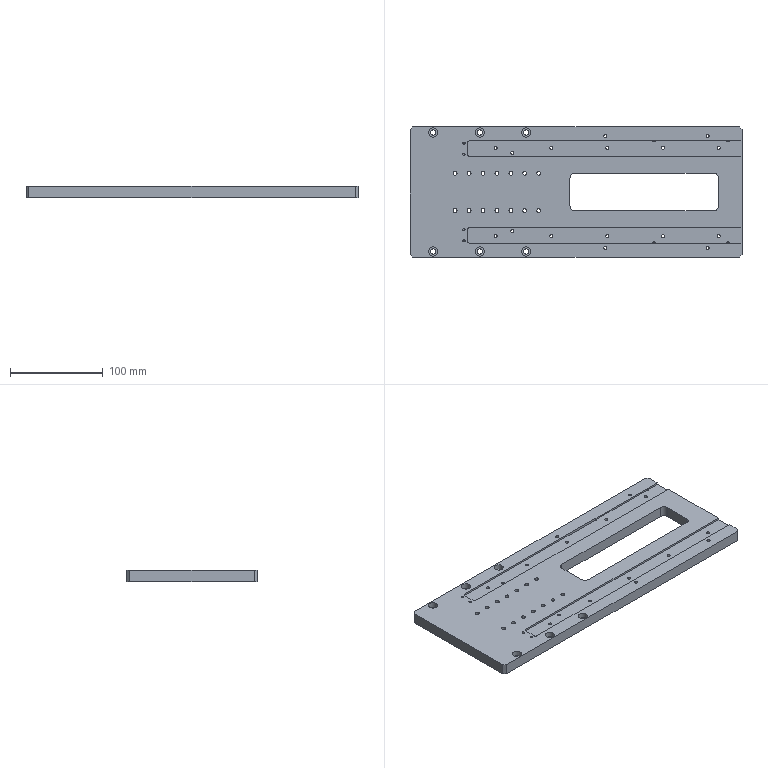Part | 1 solid | 105 faces | box 357 x 140 x 12 mm | volume 494523 mm3 | cylinder 63 | plane 42 | commonest cylinder face diameters 3.3 x16 4.2 x16 2.5 x8 5.5 x6 9.9 x6 4 x4